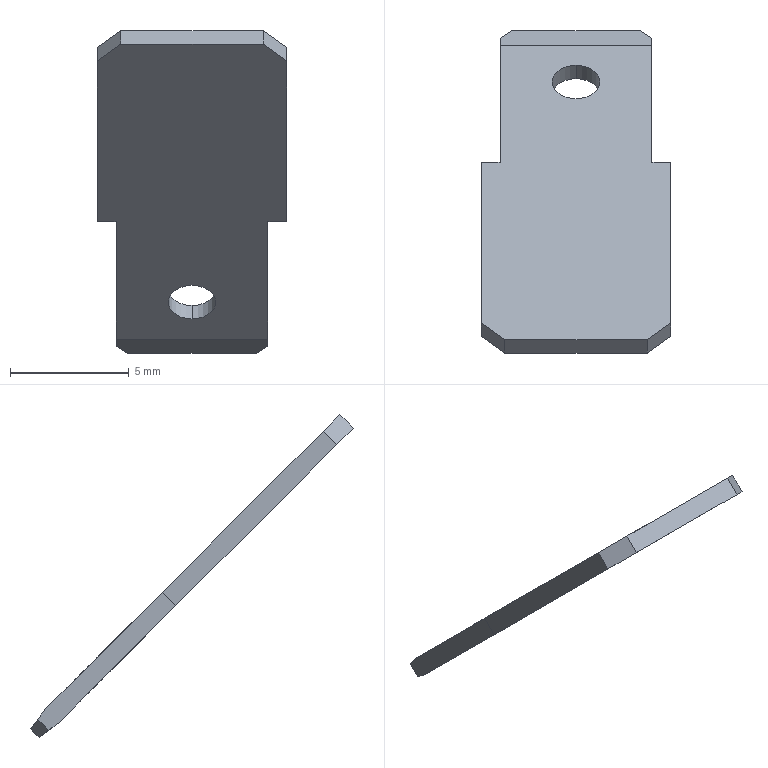Part | STEP file | DZ250_3_1_1_1 | 1 solid | 18 faces | box 8 x 13.602 x 13.602 mm | volume 104.298 mm3 | plane 16 | cylinder 2 | commonest cylinder face diameters 2 x2
STEP:
#1=CARTESIAN_POINT('',(0.,0.,0.));
#2=DIRECTION('',(0.,0.,1.));
#3=DIRECTION('',(1.,0.,0.));
#4=AXIS2_PLACEMENT_3D('',#1,#2,#3);
#5=CARTESIAN_POINT('',(0.,-5.364,5.364));
#6=VERTEX_POINT('',#5);
#7=CARTESIAN_POINT('',(0.,-5.93,4.798));
#8=VERTEX_POINT('',#7);
#9=CARTESIAN_POINT('',(0.,-5.364,5.364));
#10=DIRECTION('',(0.,-0.7071,-0.7071));
#11=VECTOR('',#10,0.8);
#12=LINE('',#9,#11);
#13=EDGE_CURVE('',#6,#8,#12,.T.);
#14=ORIENTED_EDGE('',*,*,#13,.T.);
#15=CARTESIAN_POINT('',(0.,0.8485,-1.98));
#16=VERTEX_POINT('',#15);
#17=CARTESIAN_POINT('',(0.,-5.93,4.798));
#18=DIRECTION('',(0.,0.7071,-0.7071));
#19=VECTOR('',#18,9.586);
#20=LINE('',#17,#19);
#21=EDGE_CURVE('',#8,#16,#20,.T.);
#22=ORIENTED_EDGE('',*,*,#21,.T.);
#23=CARTESIAN_POINT('',(0.,1.414,-1.414));
#24=VERTEX_POINT('',#23);
#25=CARTESIAN_POINT('',(0.,0.8485,-1.98));
#26=DIRECTION('',(0.,0.7071,0.7071));
#27=VECTOR('',#26,0.8);
#28=LINE('',#25,#27);
#29=EDGE_CURVE('',#16,#24,#28,.T.);
#30=ORIENTED_EDGE('',*,*,#29,.T.);
#31=CARTESIAN_POINT('',(0.,1.414,-1.414));
#32=DIRECTION('',(0.,-0.7071,0.7071));
#33=VECTOR('',#32,9.586);
#34=LINE('',#31,#33);
#35=EDGE_CURVE('',#24,#6,#34,.T.);
#36=ORIENTED_EDGE('',*,*,#35,.T.);
#37=EDGE_LOOP('',(#14,#22,#30,#36));
#38=FACE_OUTER_BOUND('',#37,.F.);
#39=CARTESIAN_POINT('',(0.,0.,0.));
#40=DIRECTION('',(1.,0.,0.));
#41=DIRECTION('',(0.,-1.,0.));
#42=AXIS2_PLACEMENT_3D('',#39,#40,#41);
#43=PLANE('',#42);
#44=ADVANCED_FACE('',(#38),#43,.F.);
#45=CARTESIAN_POINT('',(1.,-6.071,6.071));
#46=VERTEX_POINT('',#45);
#47=CARTESIAN_POINT('',(1.,-6.071,6.071));
#48=DIRECTION('',(-0.7071,0.5,-0.5));
#49=VECTOR('',#48,1.414);
#50=LINE('',#47,#49);
#51=EDGE_CURVE('',#46,#6,#50,.T.);
#52=ORIENTED_EDGE('',*,*,#51,.F.);
#53=CARTESIAN_POINT('',(1.,-6.637,5.505));
#54=VERTEX_POINT('',#53);
#55=CARTESIAN_POINT('',(1.,-6.637,5.505));
#56=DIRECTION('',(0.,0.7071,0.7071));
#57=VECTOR('',#56,0.8);
#58=LINE('',#55,#57);
#59=EDGE_CURVE('',#54,#46,#58,.T.);
#60=ORIENTED_EDGE('',*,*,#59,.F.);
#61=CARTESIAN_POINT('',(0.,-5.93,4.798));
#62=DIRECTION('',(0.7071,-0.5,0.5));
#63=VECTOR('',#62,1.414);
#64=LINE('',#61,#63);
#65=EDGE_CURVE('',#8,#54,#64,.T.);
#66=ORIENTED_EDGE('',*,*,#65,.F.);
#67=ORIENTED_EDGE('',*,*,#13,.F.);
#68=EDGE_LOOP('',(#52,#60,#66,#67));
#69=FACE_OUTER_BOUND('',#68,.F.);
#70=CARTESIAN_POINT('',(0.5,-6.,5.435));
#71=DIRECTION('',(-0.7071,-0.5,0.5));
#72=DIRECTION('',(0.7071,-0.5,0.5));
#73=AXIS2_PLACEMENT_3D('',#70,#71,#72);
#74=PLANE('',#73);
#75=ADVANCED_FACE('',(#69),#74,.T.);
#76=CARTESIAN_POINT('',(8.,-5.364,5.364));
#77=VERTEX_POINT('',#76);
#78=CARTESIAN_POINT('',(7.,-6.071,6.071));
#79=VERTEX_POINT('',#78);
#80=CARTESIAN_POINT('',(8.,-5.364,5.364));
#81=DIRECTION('',(-0.7071,-0.5,0.5));
#82=VECTOR('',#81,1.414);
#83=LINE('',#80,#82);
#84=EDGE_CURVE('',#77,#79,#83,.T.);
#85=ORIENTED_EDGE('',*,*,#84,.T.);
#86=CARTESIAN_POINT('',(7.,-6.071,6.071));
#87=DIRECTION('',(-1.,0.,0.));
#88=VECTOR('',#87,6.);
#89=LINE('',#86,#88);
#90=EDGE_CURVE('',#79,#46,#89,.T.);
#91=ORIENTED_EDGE('',*,*,#90,.T.);
#92=ORIENTED_EDGE('',*,*,#51,.T.);
#93=ORIENTED_EDGE('',*,*,#35,.F.);
#94=CARTESIAN_POINT('',(0.8,1.414,-1.414));
#95=VERTEX_POINT('',#94);
#96=CARTESIAN_POINT('',(0.,1.414,-1.414));
#97=DIRECTION('',(1.,0.,0.));
#98=VECTOR('',#97,0.8);
#99=LINE('',#96,#98);
#100=EDGE_CURVE('',#24,#95,#99,.T.);
#101=ORIENTED_EDGE('',*,*,#100,.T.);
#102=CARTESIAN_POINT('',(0.8,6.364,-6.364));
#103=VERTEX_POINT('',#102);
#104=CARTESIAN_POINT('',(0.8,6.364,-6.364));
#105=DIRECTION('',(0.,-0.7071,0.7071));
#106=VECTOR('',#105,7.);
#107=LINE('',#104,#106);
#108=EDGE_CURVE('',#103,#95,#107,.T.);
#109=ORIENTED_EDGE('',*,*,#108,.F.);
#110=CARTESIAN_POINT('',(7.2,6.364,-6.364));
#111=VERTEX_POINT('',#110);
#112=CARTESIAN_POINT('',(7.2,6.364,-6.364));
#113=DIRECTION('',(-1.,0.,0.));
#114=VECTOR('',#113,6.4);
#115=LINE('',#112,#114);
#116=EDGE_CURVE('',#111,#103,#115,.T.);
#117=ORIENTED_EDGE('',*,*,#116,.F.);
#118=CARTESIAN_POINT('',(7.2,1.414,-1.414));
#119=VERTEX_POINT('',#118);
#120=CARTESIAN_POINT('',(7.2,6.364,-6.364));
#121=DIRECTION('',(0.,-0.7071,0.7071));
#122=VECTOR('',#121,7.);
#123=LINE('',#120,#122);
#124=EDGE_CURVE('',#111,#119,#123,.T.);
#125=ORIENTED_EDGE('',*,*,#124,.T.);
#126=CARTESIAN_POINT('',(8.,1.414,-1.414));
#127=VERTEX_POINT('',#126);
#128=CARTESIAN_POINT('',(8.,1.414,-1.414));
#129=DIRECTION('',(-1.,0.,0.));
#130=VECTOR('',#129,0.8);
#131=LINE('',#128,#130);
#132=EDGE_CURVE('',#127,#119,#131,.T.);
#133=ORIENTED_EDGE('',*,*,#132,.F.);
#134=CARTESIAN_POINT('',(8.,-5.364,5.364));
#135=DIRECTION('',(0.,0.7071,-0.7071));
#136=VECTOR('',#135,9.586);
#137=LINE('',#134,#136);
#138=EDGE_CURVE('',#77,#127,#137,.T.);
#139=ORIENTED_EDGE('',*,*,#138,.F.);
#140=EDGE_LOOP('',(#85,#91,#92,#93,#101,#109,#117,#125,#133,#139));
#141=FACE_OUTER_BOUND('',#140,.F.);
#142=CARTESIAN_POINT('',(4.,5.515,-5.515));
#143=VERTEX_POINT('',#142);
#144=CARTESIAN_POINT('',(4.,4.101,-4.101));
#145=VERTEX_POINT('',#144);
#146=CARTESIAN_POINT('',(4.,4.808,-4.808));
#147=DIRECTION('',(0.,0.7071,0.7071));
#148=DIRECTION('',(0.,0.7071,-0.7071));
#149=AXIS2_PLACEMENT_3D('',#146,#147,#148);
#150=CIRCLE('',#149,1.);
#151=EDGE_CURVE('',#143,#145,#150,.T.);
#152=ORIENTED_EDGE('',*,*,#151,.T.);
#153=CARTESIAN_POINT('',(4.,4.808,-4.808));
#154=DIRECTION('',(0.,0.7071,0.7071));
#155=DIRECTION('',(0.,-0.7071,0.7071));
#156=AXIS2_PLACEMENT_3D('',#153,#154,#155);
#157=CIRCLE('',#156,1.);
#158=EDGE_CURVE('',#145,#143,#157,.T.);
#159=ORIENTED_EDGE('',*,*,#158,.T.);
#160=EDGE_LOOP('',(#152,#159));
#161=FACE_BOUND('',#160,.F.);
#162=CARTESIAN_POINT('',(0.,7.071,-7.071));
#163=DIRECTION('',(0.,0.7071,0.7071));
#164=DIRECTION('',(0.,-0.7071,0.7071));
#165=AXIS2_PLACEMENT_3D('',#162,#163,#164);
#166=PLANE('',#165);
#167=ADVANCED_FACE('',(#141,#161),#166,.T.);
#168=CARTESIAN_POINT('',(7.,-6.637,5.505));
#169=VERTEX_POINT('',#168);
#170=CARTESIAN_POINT('',(8.,-5.93,4.798));
#171=VERTEX_POINT('',#170);
#172=CARTESIAN_POINT('',(7.,-6.637,5.505));
#173=DIRECTION('',(0.7071,0.5,-0.5));
#174=VECTOR('',#173,1.414);
#175=LINE('',#172,#174);
#176=EDGE_CURVE('',#169,#171,#175,.T.);
#177=ORIENTED_EDGE('',*,*,#176,.F.);
#178=CARTESIAN_POINT('',(7.,-6.071,6.071));
#179=DIRECTION('',(0.,-0.7071,-0.7071));
#180=VECTOR('',#179,0.8);
#181=LINE('',#178,#180);
#182=EDGE_CURVE('',#79,#169,#181,.T.);
#183=ORIENTED_EDGE('',*,*,#182,.F.);
#184=ORIENTED_EDGE('',*,*,#84,.F.);
#185=CARTESIAN_POINT('',(8.,-5.93,4.798));
#186=DIRECTION('',(0.,0.7071,0.7071));
#187=VECTOR('',#186,0.8);
#188=LINE('',#185,#187);
#189=EDGE_CURVE('',#171,#77,#188,.T.);
#190=ORIENTED_EDGE('',*,*,#189,.F.);
#191=EDGE_LOOP('',(#177,#183,#184,#190));
#192=FACE_OUTER_BOUND('',#191,.F.);
#193=CARTESIAN_POINT('',(7.5,-6.,5.435));
#194=DIRECTION('',(0.7071,-0.5,0.5));
#195=DIRECTION('',(-0.7071,-0.5,0.5));
#196=AXIS2_PLACEMENT_3D('',#193,#194,#195);
#197=PLANE('',#196);
#198=ADVANCED_FACE('',(#192),#197,.T.);
#199=ORIENTED_EDGE('',*,*,#176,.T.);
#200=CARTESIAN_POINT('',(8.,0.8485,-1.98));
#201=VERTEX_POINT('',#200);
#202=CARTESIAN_POINT('',(8.,0.8485,-1.98));
#203=DIRECTION('',(0.,-0.7071,0.7071));
#204=VECTOR('',#203,9.586);
#205=LINE('',#202,#204);
#206=EDGE_CURVE('',#201,#171,#205,.T.);
#207=ORIENTED_EDGE('',*,*,#206,.F.);
#208=CARTESIAN_POINT('',(7.2,0.8485,-1.98));
#209=VERTEX_POINT('',#208);
#210=CARTESIAN_POINT('',(8.,0.8485,-1.98));
#211=DIRECTION('',(-1.,0.,0.));
#212=VECTOR('',#211,0.8);
#213=LINE('',#210,#212);
#214=EDGE_CURVE('',#201,#209,#213,.T.);
#215=ORIENTED_EDGE('',*,*,#214,.T.);
#216=CARTESIAN_POINT('',(7.2,5.798,-6.93));
#217=VERTEX_POINT('',#216);
#218=CARTESIAN_POINT('',(7.2,5.798,-6.93));
#219=DIRECTION('',(0.,-0.7071,0.7071));
#220=VECTOR('',#219,7.);
#221=LINE('',#218,#220);
#222=EDGE_CURVE('',#217,#209,#221,.T.);
#223=ORIENTED_EDGE('',*,*,#222,.F.);
#224=CARTESIAN_POINT('',(0.8,5.798,-6.93));
#225=VERTEX_POINT('',#224);
#226=CARTESIAN_POINT('',(7.2,5.798,-6.93));
#227=DIRECTION('',(-1.,0.,0.));
#228=VECTOR('',#227,6.4);
#229=LINE('',#226,#228);
#230=EDGE_CURVE('',#217,#225,#229,.T.);
#231=ORIENTED_EDGE('',*,*,#230,.T.);
#232=CARTESIAN_POINT('',(0.8,0.8485,-1.98));
#233=VERTEX_POINT('',#232);
#234=CARTESIAN_POINT('',(0.8,5.798,-6.93));
#235=DIRECTION('',(0.,-0.7071,0.7071));
#236=VECTOR('',#235,7.);
#237=LINE('',#234,#236);
#238=EDGE_CURVE('',#225,#233,#237,.T.);
#239=ORIENTED_EDGE('',*,*,#238,.T.);
#240=CARTESIAN_POINT('',(0.,0.8485,-1.98));
#241=DIRECTION('',(1.,0.,0.));
#242=VECTOR('',#241,0.8);
#243=LINE('',#240,#242);
#244=EDGE_CURVE('',#16,#233,#243,.T.);
#245=ORIENTED_EDGE('',*,*,#244,.F.);
#246=ORIENTED_EDGE('',*,*,#21,.F.);
#247=ORIENTED_EDGE('',*,*,#65,.T.);
#248=CARTESIAN_POINT('',(7.,-6.637,5.505));
#249=DIRECTION('',(-1.,0.,0.));
#250=VECTOR('',#249,6.);
#251=LINE('',#248,#250);
#252=EDGE_CURVE('',#169,#54,#251,.T.);
#253=ORIENTED_EDGE('',*,*,#252,.F.);
#254=EDGE_LOOP('',(#199,#207,#215,#223,#231,#239,#245,#246,#247,#253));
#255=FACE_OUTER_BOUND('',#254,.F.);
#256=CARTESIAN_POINT('',(4.,3.536,-4.667));
#257=VERTEX_POINT('',#256);
#258=CARTESIAN_POINT('',(4.,4.95,-6.081));
#259=VERTEX_POINT('',#258);
#260=CARTESIAN_POINT('',(4.,4.243,-5.374));
#261=DIRECTION('',(0.,-0.7071,-0.7071));
#262=DIRECTION('',(0.,-0.7071,0.7071));
#263=AXIS2_PLACEMENT_3D('',#260,#261,#262);
#264=CIRCLE('',#263,1.);
#265=EDGE_CURVE('',#257,#259,#264,.T.);
#266=ORIENTED_EDGE('',*,*,#265,.T.);
#267=CARTESIAN_POINT('',(4.,4.243,-5.374));
#268=DIRECTION('',(0.,-0.7071,-0.7071));
#269=DIRECTION('',(0.,0.7071,-0.7071));
#270=AXIS2_PLACEMENT_3D('',#267,#268,#269);
#271=CIRCLE('',#270,1.);
#272=EDGE_CURVE('',#259,#257,#271,.T.);
#273=ORIENTED_EDGE('',*,*,#272,.T.);
#274=EDGE_LOOP('',(#266,#273));
#275=FACE_BOUND('',#274,.F.);
#276=CARTESIAN_POINT('',(0.,-0.3314,-0.8));
#277=DIRECTION('',(0.,-0.7071,-0.7071));
#278=DIRECTION('',(0.,0.7071,-0.7071));
#279=AXIS2_PLACEMENT_3D('',#276,#277,#278);
#280=PLANE('',#279);
#281=ADVANCED_FACE('',(#255,#275),#280,.T.);
#282=ORIENTED_EDGE('',*,*,#189,.T.);
#283=ORIENTED_EDGE('',*,*,#138,.T.);
#284=CARTESIAN_POINT('',(8.,1.414,-1.414));
#285=DIRECTION('',(0.,-0.7071,-0.7071));
#286=VECTOR('',#285,0.8);
#287=LINE('',#284,#286);
#288=EDGE_CURVE('',#127,#201,#287,.T.);
#289=ORIENTED_EDGE('',*,*,#288,.T.);
#290=ORIENTED_EDGE('',*,*,#206,.T.);
#291=EDGE_LOOP('',(#282,#283,#289,#290));
#292=FACE_OUTER_BOUND('',#291,.F.);
#293=CARTESIAN_POINT('',(8.,0.,0.));
#294=DIRECTION('',(1.,0.,0.));
#295=DIRECTION('',(0.,-1.,0.));
#296=AXIS2_PLACEMENT_3D('',#293,#294,#295);
#297=PLANE('',#296);
#298=ADVANCED_FACE('',(#292),#297,.T.);
#299=ORIENTED_EDGE('',*,*,#288,.F.);
#300=ORIENTED_EDGE('',*,*,#132,.T.);
#301=CARTESIAN_POINT('',(7.2,0.8485,-1.98));
#302=DIRECTION('',(0.,0.7071,0.7071));
#303=VECTOR('',#302,0.8);
#304=LINE('',#301,#303);
#305=EDGE_CURVE('',#209,#119,#304,.T.);
#306=ORIENTED_EDGE('',*,*,#305,.F.);
#307=ORIENTED_EDGE('',*,*,#214,.F.);
#308=EDGE_LOOP('',(#299,#300,#306,#307));
#309=FACE_OUTER_BOUND('',#308,.F.);
#310=CARTESIAN_POINT('',(8.,0.8485,-1.98));
#311=DIRECTION('',(0.,-0.7071,0.7071));
#312=DIRECTION('',(-1.,0.,0.));
#313=AXIS2_PLACEMENT_3D('',#310,#311,#312);
#314=PLANE('',#313);
#315=ADVANCED_FACE('',(#309),#314,.F.);
#316=CARTESIAN_POINT('',(7.2,6.664,-6.771));
#317=VERTEX_POINT('',#316);
#318=CARTESIAN_POINT('',(7.2,6.364,-6.364));
#319=DIRECTION('',(0.,0.5944,-0.8042));
#320=VECTOR('',#319,0.5056);
#321=LINE('',#318,#320);
#322=EDGE_CURVE('',#111,#317,#321,.T.);
#323=ORIENTED_EDGE('',*,*,#322,.T.);
#324=CARTESIAN_POINT('',(7.2,6.205,-7.23));
#325=VERTEX_POINT('',#324);
#326=CARTESIAN_POINT('',(7.2,6.664,-6.771));
#327=DIRECTION('',(0.,-0.7071,-0.7071));
#328=VECTOR('',#327,0.65);
#329=LINE('',#326,#328);
#330=EDGE_CURVE('',#317,#325,#329,.T.);
#331=ORIENTED_EDGE('',*,*,#330,.T.);
#332=CARTESIAN_POINT('',(7.2,6.205,-7.23));
#333=DIRECTION('',(0.,-0.8042,0.5944));
#334=VECTOR('',#333,0.5056);
#335=LINE('',#332,#334);
#336=EDGE_CURVE('',#325,#217,#335,.T.);
#337=ORIENTED_EDGE('',*,*,#336,.T.);
#338=ORIENTED_EDGE('',*,*,#222,.T.);
#339=ORIENTED_EDGE('',*,*,#305,.T.);
#340=ORIENTED_EDGE('',*,*,#124,.F.);
#341=EDGE_LOOP('',(#323,#331,#337,#338,#339,#340));
#342=FACE_OUTER_BOUND('',#341,.F.);
#343=CARTESIAN_POINT('',(7.2,0.8485,-1.98));
#344=DIRECTION('',(-1.,0.,0.));
#345=DIRECTION('',(0.,0.7071,-0.7071));
#346=AXIS2_PLACEMENT_3D('',#343,#344,#345);
#347=PLANE('',#346);
#348=ADVANCED_FACE('',(#342),#347,.F.);
#349=CARTESIAN_POINT('',(0.8,6.664,-6.771));
#350=VERTEX_POINT('',#349);
#351=CARTESIAN_POINT('',(0.8,6.664,-6.771));
#352=DIRECTION('',(0.,-0.5944,0.8042));
#353=VECTOR('',#352,0.5056);
#354=LINE('',#351,#353);
#355=EDGE_CURVE('',#350,#103,#354,.T.);
#356=ORIENTED_EDGE('',*,*,#355,.F.);
#357=CARTESIAN_POINT('',(1.3,6.965,-7.177));
#358=VERTEX_POINT('',#357);
#359=CARTESIAN_POINT('',(0.8,6.664,-6.771));
#360=DIRECTION('',(0.7032,0.4226,-0.5718));
#361=VECTOR('',#360,0.7111);
#362=LINE('',#359,#361);
#363=EDGE_CURVE('',#350,#358,#362,.T.);
#364=ORIENTED_EDGE('',*,*,#363,.T.);
#365=CARTESIAN_POINT('',(6.7,6.965,-7.177));
#366=VERTEX_POINT('',#365);
#367=CARTESIAN_POINT('',(6.7,6.965,-7.177));
#368=DIRECTION('',(-1.,0.,0.));
#369=VECTOR('',#368,5.4);
#370=LINE('',#367,#369);
#371=EDGE_CURVE('',#366,#358,#370,.T.);
#372=ORIENTED_EDGE('',*,*,#371,.F.);
#373=CARTESIAN_POINT('',(6.7,6.965,-7.177));
#374=DIRECTION('',(0.7032,-0.4226,0.5718));
#375=VECTOR('',#374,0.7111);
#376=LINE('',#373,#375);
#377=EDGE_CURVE('',#366,#317,#376,.T.);
#378=ORIENTED_EDGE('',*,*,#377,.T.);
#379=ORIENTED_EDGE('',*,*,#322,.F.);
#380=ORIENTED_EDGE('',*,*,#116,.T.);
#381=EDGE_LOOP('',(#356,#364,#372,#378,#379,#380));
#382=FACE_OUTER_BOUND('',#381,.F.);
#383=CARTESIAN_POINT('',(4.,6.664,-6.771));
#384=DIRECTION('',(0.,0.8042,0.5944));
#385=DIRECTION('',(0.,0.5944,-0.8042));
#386=AXIS2_PLACEMENT_3D('',#383,#384,#385);
#387=PLANE('',#386);
#388=ADVANCED_FACE('',(#382),#387,.T.);
#389=ORIENTED_EDGE('',*,*,#355,.T.);
#390=ORIENTED_EDGE('',*,*,#108,.T.);
#391=CARTESIAN_POINT('',(0.8,0.8485,-1.98));
#392=DIRECTION('',(0.,0.7071,0.7071));
#393=VECTOR('',#392,0.8);
#394=LINE('',#391,#393);
#395=EDGE_CURVE('',#233,#95,#394,.T.);
#396=ORIENTED_EDGE('',*,*,#395,.F.);
#397=ORIENTED_EDGE('',*,*,#238,.F.);
#398=CARTESIAN_POINT('',(0.8,6.205,-7.23));
#399=VERTEX_POINT('',#398);
#400=CARTESIAN_POINT('',(0.8,5.798,-6.93));
#401=DIRECTION('',(0.,0.8042,-0.5944));
#402=VECTOR('',#401,0.5056);
#403=LINE('',#400,#402);
#404=EDGE_CURVE('',#225,#399,#403,.T.);
#405=ORIENTED_EDGE('',*,*,#404,.T.);
#406=CARTESIAN_POINT('',(0.8,6.205,-7.23));
#407=DIRECTION('',(0.,0.7071,0.7071));
#408=VECTOR('',#407,0.65);
#409=LINE('',#406,#408);
#410=EDGE_CURVE('',#399,#350,#409,.T.);
#411=ORIENTED_EDGE('',*,*,#410,.T.);
#412=EDGE_LOOP('',(#389,#390,#396,#397,#405,#411));
#413=FACE_OUTER_BOUND('',#412,.F.);
#414=CARTESIAN_POINT('',(0.8,6.505,-7.637));
#415=DIRECTION('',(1.,0.,0.));
#416=DIRECTION('',(0.,-0.7071,0.7071));
#417=AXIS2_PLACEMENT_3D('',#414,#415,#416);
#418=PLANE('',#417);
#419=ADVANCED_FACE('',(#413),#418,.F.);
#420=ORIENTED_EDGE('',*,*,#29,.F.);
#421=ORIENTED_EDGE('',*,*,#244,.T.);
#422=ORIENTED_EDGE('',*,*,#395,.T.);
#423=ORIENTED_EDGE('',*,*,#100,.F.);
#424=EDGE_LOOP('',(#420,#421,#422,#423));
#425=FACE_OUTER_BOUND('',#424,.F.);
#426=CARTESIAN_POINT('',(0.8,0.8485,-1.98));
#427=DIRECTION('',(0.,-0.7071,0.7071));
#428=DIRECTION('',(-1.,0.,0.));
#429=AXIS2_PLACEMENT_3D('',#426,#427,#428);
#430=PLANE('',#429);
#431=ADVANCED_FACE('',(#425),#430,.F.);
#432=CARTESIAN_POINT('',(1.3,6.611,-7.531));
#433=VERTEX_POINT('',#432);
#434=CARTESIAN_POINT('',(1.3,6.611,-7.531));
#435=DIRECTION('',(-0.7032,-0.5718,0.4226));
#436=VECTOR('',#435,0.7111);
#437=LINE('',#434,#436);
#438=EDGE_CURVE('',#433,#399,#437,.T.);
#439=ORIENTED_EDGE('',*,*,#438,.T.);
#440=ORIENTED_EDGE('',*,*,#404,.F.);
#441=ORIENTED_EDGE('',*,*,#230,.F.);
#442=ORIENTED_EDGE('',*,*,#336,.F.);
#443=CARTESIAN_POINT('',(6.7,6.611,-7.531));
#444=VERTEX_POINT('',#443);
#445=CARTESIAN_POINT('',(7.2,6.205,-7.23));
#446=DIRECTION('',(-0.7032,0.5718,-0.4226));
#447=VECTOR('',#446,0.7111);
#448=LINE('',#445,#447);
#449=EDGE_CURVE('',#325,#444,#448,.T.);
#450=ORIENTED_EDGE('',*,*,#449,.T.);
#451=CARTESIAN_POINT('',(6.7,6.611,-7.531));
#452=DIRECTION('',(-1.,0.,0.));
#453=VECTOR('',#452,5.4);
#454=LINE('',#451,#453);
#455=EDGE_CURVE('',#444,#433,#454,.T.);
#456=ORIENTED_EDGE('',*,*,#455,.T.);
#457=EDGE_LOOP('',(#439,#440,#441,#442,#450,#456));
#458=FACE_OUTER_BOUND('',#457,.F.);
#459=CARTESIAN_POINT('',(4.,6.205,-7.23));
#460=DIRECTION('',(0.,-0.5944,-0.8042));
#461=DIRECTION('',(0.,-0.8042,0.5944));
#462=AXIS2_PLACEMENT_3D('',#459,#460,#461);
#463=PLANE('',#462);
#464=ADVANCED_FACE('',(#458),#463,.T.);
#465=ORIENTED_EDGE('',*,*,#363,.F.);
#466=ORIENTED_EDGE('',*,*,#410,.F.);
#467=ORIENTED_EDGE('',*,*,#438,.F.);
#468=CARTESIAN_POINT('',(1.3,6.611,-7.531));
#469=DIRECTION('',(0.,0.7071,0.7071));
#470=VECTOR('',#469,0.5);
#471=LINE('',#468,#470);
#472=EDGE_CURVE('',#433,#358,#471,.T.);
#473=ORIENTED_EDGE('',*,*,#472,.T.);
#474=EDGE_LOOP('',(#465,#466,#467,#473));
#475=FACE_OUTER_BOUND('',#474,.F.);
#476=CARTESIAN_POINT('',(1.05,6.611,-7.177));
#477=DIRECTION('',(-0.7071,0.5,-0.5));
#478=DIRECTION('',(-0.7071,-0.5,0.5));
#479=AXIS2_PLACEMENT_3D('',#476,#477,#478);
#480=PLANE('',#479);
#481=ADVANCED_FACE('',(#475),#480,.T.);
#482=ORIENTED_EDGE('',*,*,#371,.T.);
#483=ORIENTED_EDGE('',*,*,#472,.F.);
#484=ORIENTED_EDGE('',*,*,#455,.F.);
#485=CARTESIAN_POINT('',(6.7,6.965,-7.177));
#486=DIRECTION('',(0.,-0.7071,-0.7071));
#487=VECTOR('',#486,0.5);
#488=LINE('',#485,#487);
#489=EDGE_CURVE('',#366,#444,#488,.T.);
#490=ORIENTED_EDGE('',*,*,#489,.F.);
#491=EDGE_LOOP('',(#482,#483,#484,#490));
#492=FACE_OUTER_BOUND('',#491,.F.);
#493=CARTESIAN_POINT('',(0.,6.505,-7.637));
#494=DIRECTION('',(0.,0.7071,-0.7071));
#495=DIRECTION('',(0.,0.7071,0.7071));
#496=AXIS2_PLACEMENT_3D('',#493,#494,#495);
#497=PLANE('',#496);
#498=ADVANCED_FACE('',(#492),#497,.T.);
#499=ORIENTED_EDGE('',*,*,#377,.F.);
#500=ORIENTED_EDGE('',*,*,#489,.T.);
#501=ORIENTED_EDGE('',*,*,#449,.F.);
#502=ORIENTED_EDGE('',*,*,#330,.F.);
#503=EDGE_LOOP('',(#499,#500,#501,#502));
#504=FACE_OUTER_BOUND('',#503,.F.);
#505=CARTESIAN_POINT('',(6.95,6.611,-7.177));
#506=DIRECTION('',(0.7071,0.5,-0.5));
#507=DIRECTION('',(0.7071,-0.5,0.5));
#508=AXIS2_PLACEMENT_3D('',#505,#506,#507);
#509=PLANE('',#508);
#510=ADVANCED_FACE('',(#504),#509,.T.);
#511=ORIENTED_EDGE('',*,*,#182,.T.);
#512=ORIENTED_EDGE('',*,*,#252,.T.);
#513=ORIENTED_EDGE('',*,*,#59,.T.);
#514=ORIENTED_EDGE('',*,*,#90,.F.);
#515=EDGE_LOOP('',(#511,#512,#513,#514));
#516=FACE_OUTER_BOUND('',#515,.F.);
#517=CARTESIAN_POINT('',(8.,-6.071,6.071));
#518=DIRECTION('',(0.,-0.7071,0.7071));
#519=DIRECTION('',(0.,-0.7071,-0.7071));
#520=AXIS2_PLACEMENT_3D('',#517,#518,#519);
#521=PLANE('',#520);
#522=ADVANCED_FACE('',(#516),#521,.T.);
#523=ORIENTED_EDGE('',*,*,#265,.F.);
#524=CARTESIAN_POINT('',(4.,3.536,-4.667));
#525=DIRECTION('',(0.,0.7071,0.7071));
#526=VECTOR('',#525,0.8);
#527=LINE('',#524,#526);
#528=EDGE_CURVE('',#257,#145,#527,.T.);
#529=ORIENTED_EDGE('',*,*,#528,.T.);
#530=ORIENTED_EDGE('',*,*,#151,.F.);
#531=CARTESIAN_POINT('',(4.,4.95,-6.081));
#532=DIRECTION('',(0.,0.7071,0.7071));
#533=VECTOR('',#532,0.8);
#534=LINE('',#531,#533);
#535=EDGE_CURVE('',#259,#143,#534,.T.);
#536=ORIENTED_EDGE('',*,*,#535,.F.);
#537=EDGE_LOOP('',(#523,#529,#530,#536));
#538=FACE_OUTER_BOUND('',#537,.F.);
#539=CARTESIAN_POINT('',(4.,4.243,-5.374));
#540=DIRECTION('',(0.,-0.7071,-0.7071));
#541=DIRECTION('',(0.,-0.7071,0.7071));
#542=AXIS2_PLACEMENT_3D('',#539,#540,#541);
#543=CYLINDRICAL_SURFACE('',#542,1.);
#544=ADVANCED_FACE('',(#538),#543,.F.);
#545=ORIENTED_EDGE('',*,*,#272,.F.);
#546=ORIENTED_EDGE('',*,*,#535,.T.);
#547=ORIENTED_EDGE('',*,*,#158,.F.);
#548=ORIENTED_EDGE('',*,*,#528,.F.);
#549=EDGE_LOOP('',(#545,#546,#547,#548));
#550=FACE_OUTER_BOUND('',#549,.F.);
#551=CARTESIAN_POINT('',(4.,4.243,-5.374));
#552=DIRECTION('',(0.,-0.7071,-0.7071));
#553=DIRECTION('',(0.,-0.7071,0.7071));
#554=AXIS2_PLACEMENT_3D('',#551,#552,#553);
#555=CYLINDRICAL_SURFACE('',#554,1.);
#556=ADVANCED_FACE('',(#550),#555,.F.);
#557=CLOSED_SHELL('',(#44,#75,#167,#198,#281,#298,#315,#348,#388,#419,#431,#464,#481,#498,#510,#522,#544,#556));
#558=MANIFOLD_SOLID_BREP('',#557);
#559=(LENGTH_UNIT()NAMED_UNIT(*)SI_UNIT(.MILLI.,.METRE.));
#560=UNCERTAINTY_MEASURE_WITH_UNIT(LENGTH_MEASURE(0.00209),#559,'','');
#561=(NAMED_UNIT(*)PLANE_ANGLE_UNIT()SI_UNIT($,.RADIAN.));
#562=PLANE_ANGLE_MEASURE_WITH_UNIT(PLANE_ANGLE_MEASURE(0.01745),#561);
#563=(CONVERSION_BASED_UNIT('DEGREE',#562)NAMED_UNIT(*)PLANE_ANGLE_UNIT());
#564=(NAMED_UNIT(*)SI_UNIT($,.STERADIAN.)SOLID_ANGLE_UNIT());
#565=(GEOMETRIC_REPRESENTATION_CONTEXT(3)GLOBAL_UNCERTAINTY_ASSIGNED_CONTEXT((#560))GLOBAL_UNIT_ASSIGNED_CONTEXT((#559,#563,#564))REPRESENTATION_CONTEXT('',''));
#566=ADVANCED_BREP_SHAPE_REPRESENTATION('',(#4,#558),#565);